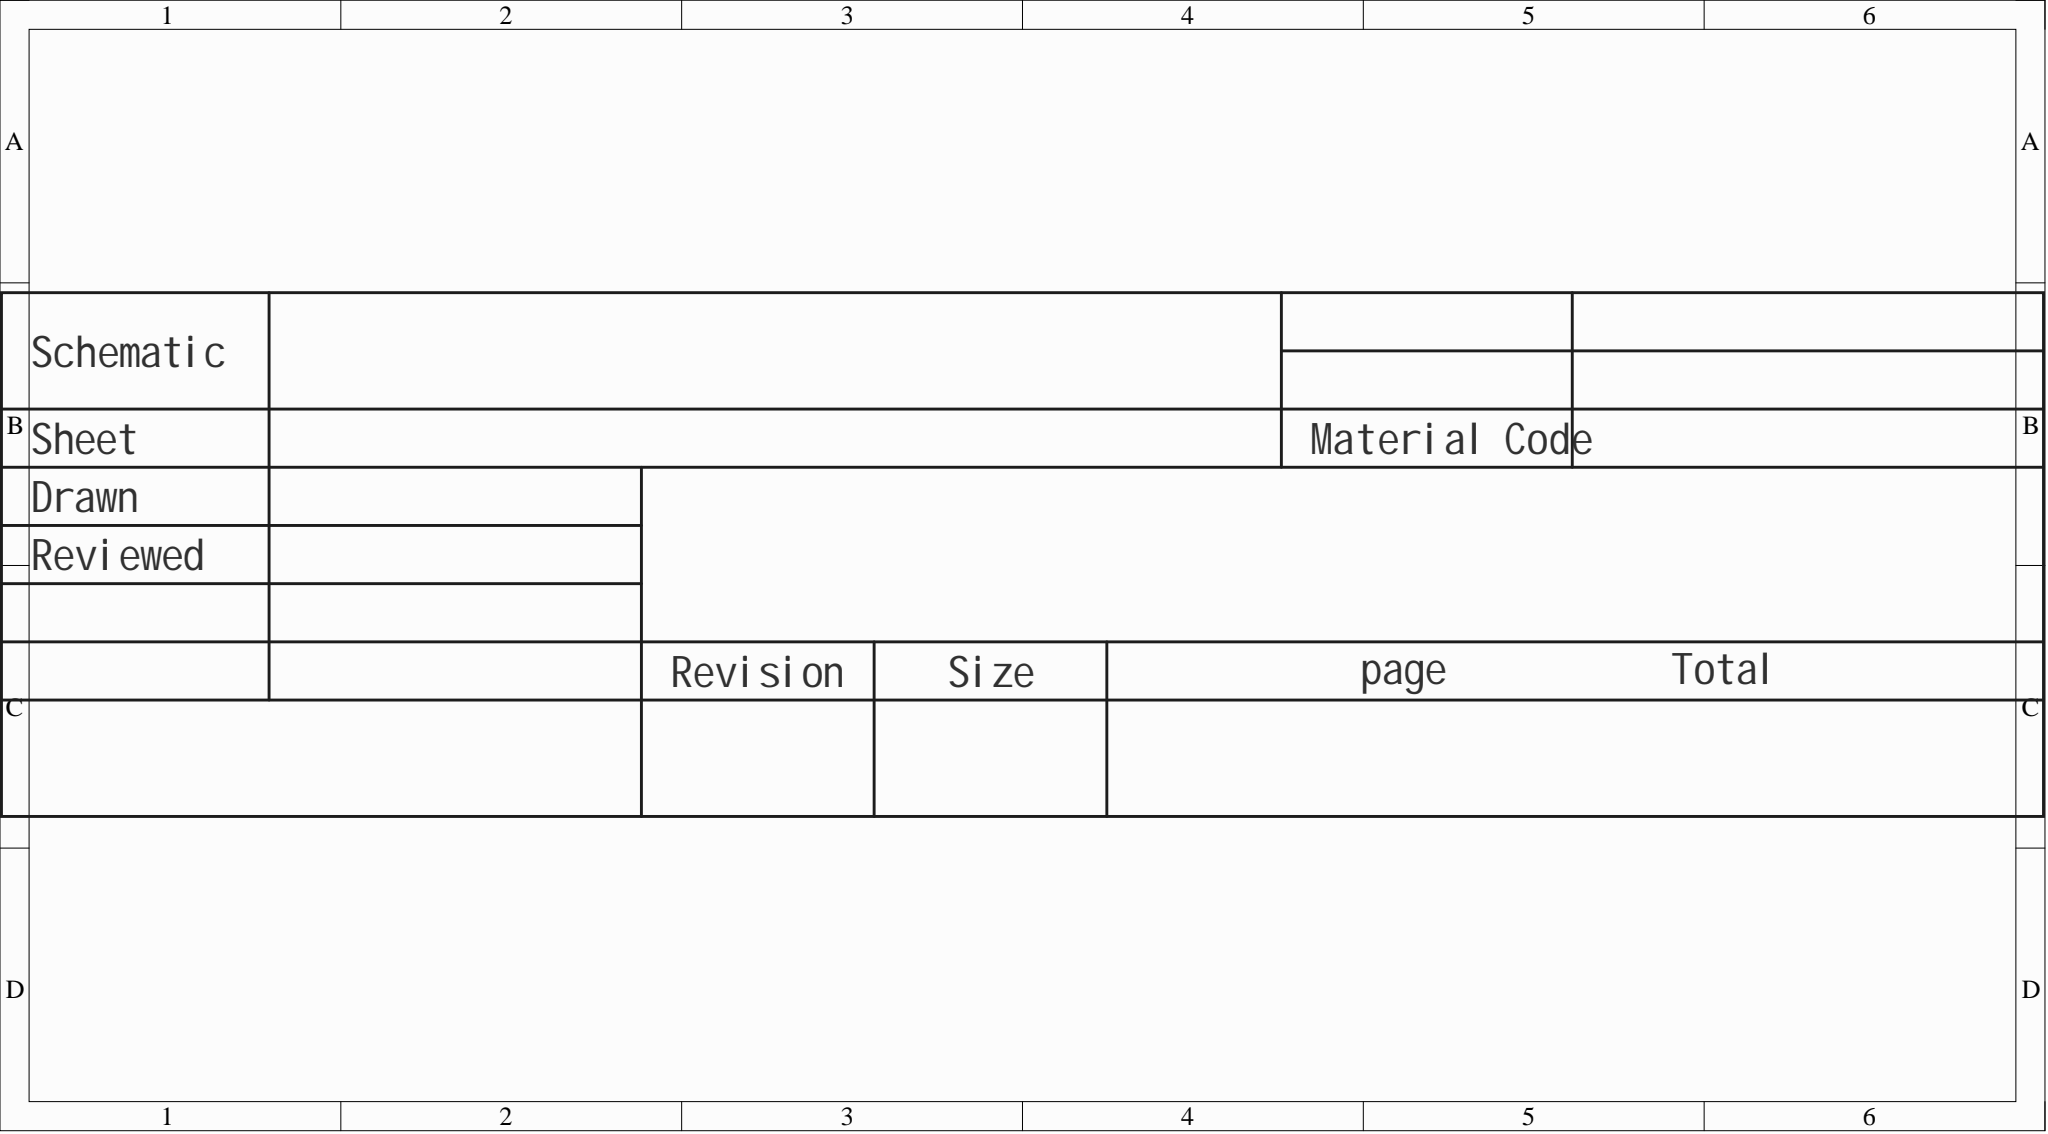Circuit board | Altium Designer | 64 parts | 96 nets
Bill of materials:
Comment,Description,Designator,Footprint,LibRef,Quantity
"buzzer","","BUZZER1","BUZ-TH_BD12.0-P6.00-D0.9-RD","buzzer","1"
"100uF","","C1","C0805","CAP_0805","1"
"10nF","","C2","C0805","CAP_0805","1"
"","","H1","HDR-TH_4P-P2.54-V-M","HDR-M_2.54_1x4P","1"
"Tact switch 3*4*H","","J2, J3, J4, J5","SW-SMD_L4.0-W2.9-LS5.0","轻触按键3*4*H","4"
"","","LED4, LED5, LED7","LED-SEG-TH_10P-L12.6-W19.0-P2.54-S15.24-BL","LED_SEG_TH_0.56x1","3"
"","","LED6, LED8, LED9","LED_TH-3mm","LED_TH-R_3mm","3"
"2N2222A","Transistor type: NPN; Collector current (Ic): 600mA; Collector-emitter breakdown voltage (Vceo): 40V; Power (Pd): 625mW; DC current gain (hFE@Ic,Vce): 40@500mA,10V;","Q1","TO-92-3_L4.9-W3.7-P1.27-L","2N2222A","1"
"10k","","R1, R28, R29, R30, R31, R32, R33, R34, R35","R0603","Res_0603","9"
"2.2k","","R2","R0603","Res_0603","1"
"330","","R36, R37, R38, R39, R40, R41, R42, R44, R45, R46, R47, R48, R49, R50, R52, R53, R54, R55, R56, R57, R58","R0603","Res_0603","21"
"500","","R59","R0603","Res_0603","1"
"2k","","R60","R0603","Res_0603","1"
"DIP switch EI-04","Type: slide, raised; Circuit: SPST; Switch positions: 4 positions; Life: -; Color: black;","SW1, SW2","SW-TH_DIPSWITCHEI-04","拨码开关EI-04","2"
"SWITCH-slide three-pin two-position","","SW3","SW-TH_C9900003112","SWITCH-拨动-三脚两档","1"
"NE555PE4","Precision timer 8-PDIP 0 to 70","U8","PDIP-8_L9.6-W6.4-P2.54-LS7.9-BL-1","NE555PE4","1"
"SN74148N","","U60","PDIP-16_L19.3-W6.4-P2.54-LS7.9-BL","SN74148N","1"
"74279N","","U62","DIP-16_L19.8-W6.5-P2.54-LS7.6-BL","XD74LS160","1"
"SN74LS48N","","U63, U70, U72","DIP-16_L19.3-W6.4-P2.54-LS7.6-BL","SN74LS48N","3"
"SN74LS00N(LX)","Logic type: NAND gate; Channels: 4; Supply voltage: 2V~6V; Quiescent current (max): 2uA; Max propagation delay: 7ns@6V;","U64","PDIP-14_L19.3-W6.4-P2.54-LS7.9-BL","SN74LS00N(LX)","1"
"SN74LS04DR","Supply voltage: 4.75V~5.25V; Circuits: 6; Max propagation delay (tpd): 15ns@5V,15pF;","U65, U71","SOIC-14_L8.7-W3.9-P1.27-LS6.0-BL","SN74LS04DR","2"
"SN74LS08DR(LX)","Logic type: AND gate; Channels: 4; Supply voltage: 2V~6V; Quiescent current (max): 2uA; Max propagation delay: 15ns@6V;","U66","SOIC-14_L8.7-W3.9-P1.27-LS6.0-BL","SN74LS08DR(LX)","1"
"SN74LS32DR","Logic type: OR gate; Channels: 4; Supply voltage: 4.75V~5.25V; Max propagation delay: 22ns@5V,15pF;","U67","SOIC-14_L8.7-W3.9-P1.27-LS6.0-BL","SN74LS32DR","1"
"SN74LS192N(LX)","Operating voltage: 2V~6V; Elements: 1; Trigger edge: rising edge; Count rate: 24MHz;","U68, U69","PDIP-16_L19.3-W6.4-P2.54-LS7.94-BL","SN74LS192N(LX)","2"
Netlist (Protel format):
[
BUZZER1
BUZ-TH_BD12.0-P6.00-D0.9-RD
buzzer



]
[
C1
C0805
100uF



]
[
C2
C0805
10nF



]
[
H1
HDR-TH_4P-P2.54-V-M




]
[
J2
SW-SMD_L4.0-W2.9-LS5.0
Tact switch 3*4*H



]
[
J3
SW-SMD_L4.0-W2.9-LS5.0
Tact switch 3*4*H



]
[
J4
SW-SMD_L4.0-W2.9-LS5.0
Tact switch 3*4*H



]
[
J5
SW-SMD_L4.0-W2.9-LS5.0
Tact switch 3*4*H



]
[
LED4
LED-SEG-TH_10P-L12.6-W19.0-P2.54-S15.24-BL




]
[
LED5
LED-SEG-TH_10P-L12.6-W19.0-P2.54-S15.24-BL




]
[
LED6
LED_TH-3mm




]
[
LED7
LED-SEG-TH_10P-L12.6-W19.0-P2.54-S15.24-BL




]
[
LED8
LED_TH-3mm




]
[
LED9
LED_TH-3mm




]
[
Q1
TO-92-3_L4.9-W3.7-P1.27-L
2N2222A



]
[
R1
R0603
10k



]
[
R2
R0603
2.2k



]
[
R28
R0603
10k



]
[
R29
R0603
10k



]
[
R30
R0603
10k



]
[
R31
R0603
10k



]
[
R32
R0603
10k



]
[
R33
R0603
10k



]
[
R34
R0603
10k



]
[
R35
R0603
10k



]
[
R36
R0603
330



]
[
R37
R0603
330



]
[
R38
R0603
330



]
[
R39
R0603
330



]
[
R40
R0603
330



]
[
R41
R0603
330



]
[
R42
R0603
330



]
[
R44
R0603
330



]
[
R45
R0603
330



]
[
R46
R0603
330



]
[
R47
R0603
330



]
[
R48
R0603
330



]
[
R49
R0603
330



]
[
R50
R0603
330



]
[
R52
R0603
330



]
[
R53
R0603
330



]
[
R54
R0603
330



]
[
R55
R0603
330



]
[
R56
R0603
330



]
[
R57
R0603
330



]
[
R58
R0603
330



]
[
R59
R0603
500



]
[
R60
R0603
2k



]
[
SW1
SW-TH_DIPSWITCHEI-04
DIP switch EI-04



]
[
SW2
SW-TH_DIPSWITCHEI-04
DIP switch EI-04



]
[
SW3
SW-TH_C9900003112
SWITCH-slide three-pin two-position



]
[
U8
PDIP-8_L9.6-W6.4-P2.54-LS7.9-BL-1
NE555PE4



]
[
U60
PDIP-16_L19.3-W6.4-P2.54-LS7.9-BL
SN74148N



]
[
U62
DIP-16_L19.8-W6.5-P2.54-LS7.6-BL
74279N



]
[
U63
DIP-16_L19.3-W6.4-P2.54-LS7.6-BL
SN74LS48N



]
[
U64
PDIP-14_L19.3-W6.4-P2.54-LS7.9-BL
SN74LS00N(LX)



]
[
U65
SOIC-14_L8.7-W3.9-P1.27-LS6.0-BL
SN74LS04DR



]
[
U66
SOIC-14_L8.7-W3.9-P1.27-LS6.0-BL
SN74LS08DR(LX)



]
[
U67
SOIC-14_L8.7-W3.9-P1.27-LS6.0-BL
SN74LS32DR



]
[
U68
PDIP-16_L19.3-W6.4-P2.54-LS7.94-BL
SN74LS192N(LX)



]
[
U69
PDIP-16_L19.3-W6.4-P2.54-LS7.94-BL
SN74LS192N(LX)



]
[
U70
DIP-16_L19.3-W6.4-P2.54-LS7.6-BL
SN74LS48N



]
[
U71
SOIC-14_L8.7-W3.9-P1.27-LS6.0-BL
SN74LS04DR



]
[
U72
DIP-16_L19.3-W6.4-P2.54-LS7.6-BL
SN74LS48N



]
(
VCC
BUZZER1-2
H1-1
H1-2
R1-2
R28-2
R29-2
R30-2
R31-2
R32-2
R33-2
R34-2
R35-2
SW1-1
SW1-2
SW1-3
SW1-4
SW2-1
SW2-2
SW2-3
SW2-4
SW3-3
U8-4
U8-8
U60-16
U63-3
U63-5
U63-16
U64-14
U65-14
U66-14
U67-14
U68-5
U68-16
U69-5
U69-16
U70-3
U70-4
U70-5
U70-16
U71-14
U72-3
U72-4
U72-5
U72-16
)
(
NetU69_7
U69-7
U72-6
)
(
NetU69_6
U69-6
U72-2
)
(
NetU69_3
U69-3
U72-7
)
(
NetU69_2
U69-2
U72-1
)
(
NetU68_13
U68-13
U71-3
)
(
NetU68_7
U68-7
U70-6
)
(
NetU68_6
U68-6
U70-2
)
(
NetU68_4
U68-4
U69-13
)
(
NetU68_3
U68-3
U70-7
)
(
NetU68_2
U68-2
U70-1
)
(
NetU66_9
U66-9
U67-3
)
(
NetU66_6
U66-6
U67-2
)
(
NetU66_3
U66-3
U67-1
)
(
NetU65_4
U65-4
U66-5
)
(
NetU64_3
U64-3
U69-4
)
(
NetU64_2
U64-2
U64-8
)
(
NetU64_1
U64-1
U64-4
U65-2
)
(
NetU62_13
U62-13
U63-4
U65-1
)
(
NetU62_9
U62-9
U63-2
)
(
NetU62_7
U62-7
U63-1
)
(
NetU62_4
U62-4
U63-7
)
(
NetU60_14
U60-14
U62-15
)
(
NetU60_9
U60-9
U62-2
U62-3
)
(
NetU60_7
U60-7
U62-6
)
(
NetU60_6
U60-6
U62-11
U62-12
)
(
NetU8_3
U8-3
U64-9
U66-10
)
(
NetSW3_2
SW3-2
U62-1
U62-5
U62-10
U62-14
U68-11
U69-11
)
(
NetSW2_8
SW2-8
U69-15
)
(
NetSW2_7
SW2-7
U69-1
)
(
NetSW2_6
SW2-6
U69-10
)
(
NetSW2_5
SW2-5
U69-9
)
(
NetSW1_8
SW1-8
U68-15
)
(
NetSW1_7
SW1-7
U68-1
)
(
NetSW1_6
SW1-6
U68-10
)
(
NetSW1_5
SW1-5
U68-9
)
(
NetR59_2
R59-2
R60-2
U66-8
)
(
NetR58_1
R58-1
U72-14
)
(
NetR57_1
R57-1
U72-15
)
(
NetR56_1
R56-1
U72-9
)
(
NetR55_1
R55-1
U72-10
)
(
NetR54_1
R54-1
U72-11
)
(
NetR53_1
R53-1
U72-12
)
(
NetR52_1
R52-1
U72-13
)
(
NetR50_1
R50-1
U70-14
)
(
NetR49_1
R49-1
U70-15
)
(
NetR48_1
R48-1
U70-9
)
(
NetR47_1
R47-1
U70-10
)
(
NetR46_1
R46-1
U70-11
)
(
NetR45_1
R45-1
U70-12
)
(
NetR44_1
R44-1
U70-13
)
(
NetR42_1
R42-1
U63-14
)
(
NetR41_1
R41-1
U63-15
)
(
NetR40_1
R40-1
U63-9
)
(
NetR39_1
R39-1
U63-10
)
(
NetR38_1
R38-1
U63-11
)
(
NetR37_1
R37-1
U63-12
)
(
NetR36_1
R36-1
U63-13
)
(
NetR35_1
R35-1
U60-10
)
(
NetR30_1
R30-1
U60-2
)
(
NetR29_1
R29-1
U60-3
)
(
NetR28_1
R28-1
U60-4
)
(
NetR1_1
R1-1
R2-2
U8-7
)
(
NetQ1_2
Q1-2
R60-1
)
(
NetLED9_1
LED9-1
U60-5
U64-6
U66-2
U66-4
)
(
NetLED8_1
LED8-1
R59-1
)
(
NetLED7_10
LED7-10
R58-2
)
(
NetLED7_9
LED7-9
R57-2
)
(
NetLED7_7
LED7-7
R52-2
)
(
NetLED7_6
LED7-6
R53-2
)
(
NetLED7_4
LED7-4
R54-2
)
(
NetLED7_2
LED7-2
R55-2
)
(
NetLED7_1
LED7-1
R56-2
)
(
NetLED6_1
LED6-1
U64-5
U64-10
U65-3
U66-1
U71-4
)
(
NetLED5_10
LED5-10
R50-2
)
(
NetLED5_9
LED5-9
R49-2
)
(
NetLED5_7
LED5-7
R44-2
)
(
NetLED5_6
LED5-6
R45-2
)
(
NetLED5_4
LED5-4
R46-2
)
(
NetLED5_2
LED5-2
R47-2
)
(
NetLED5_1
LED5-1
R48-2
)
(
NetLED4_10
LED4-10
R42-2
)
(
NetLED4_9
LED4-9
R41-2
)
(
NetLED4_7
LED4-7
R36-2
)
(
NetLED4_6
LED4-6
R37-2
)
(
NetLED4_4
LED4-4
R38-2
)
(
NetLED4_2
LED4-2
R39-2
)
(
NetLED4_1
LED4-1
R40-2
)
(
NetJ5_2
J5-2
R31-1
U60-1
)
(
NetJ4_2
J4-2
R32-1
U60-13
)
(
NetJ3_2
J3-2
R33-1
U60-12
)
(
NetJ2_2
J2-2
R34-1
U60-11
)
(
NetC2_2
C2-2
U8-5
)
(
NetC1_2
C1-2
R2-1
U8-2
U8-6
)
(
NetBUZZER1_1
BUZZER1-1
Q1-3
)
(
GND
C1-1
C2-1
H1-3
H1-4
J2-1
J3-1
J4-1
J5-1
LED6-2
LED8-2
LED9-2
Q1-1
SW3-1
U8-1
U60-8
U63-6
U63-8
U64-7
U65-7
U66-7
U67-7
U68-8
U68-14
U69-8
U69-14
U70-8
U71-7
U72-8
)